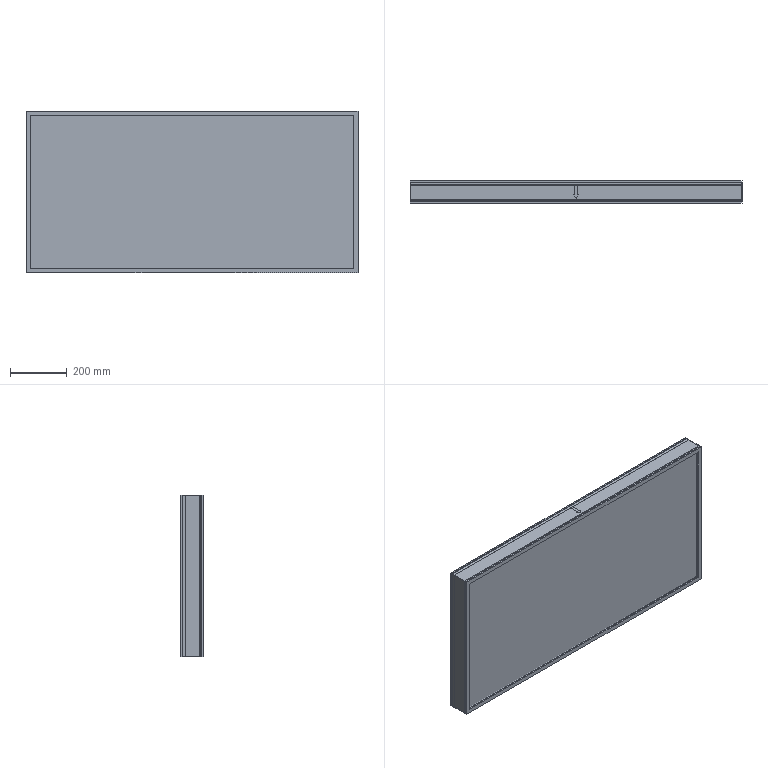Part | SolidWorks | features BaseBody 6 | 6 solids | 70 faces | box 1170 x 79 x 570 mm | volume 72868307 mm3 | plane 70